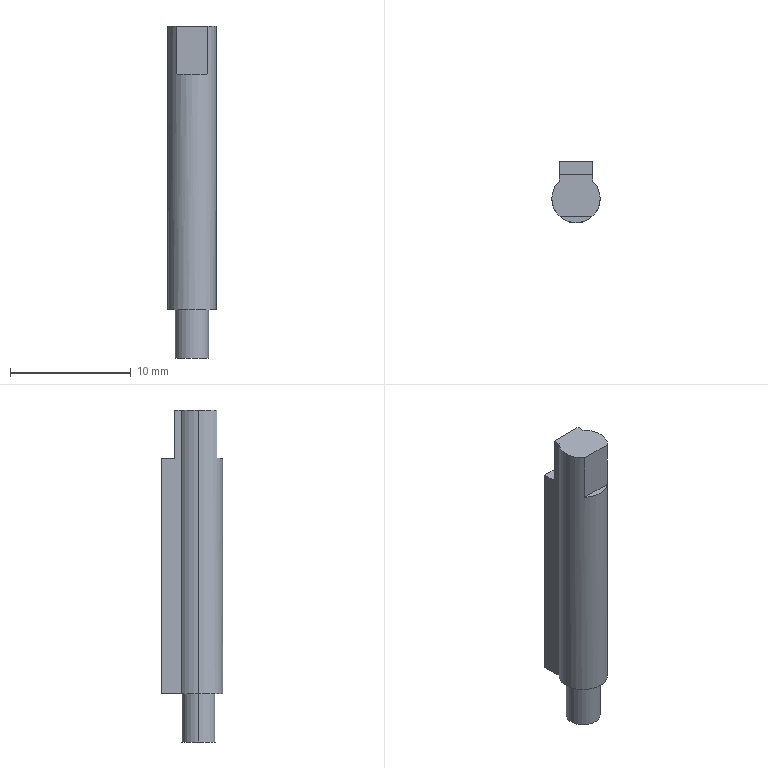Part | STEP file | QA-HI_MDX-SD_2 | 1 solid | 25 faces | box 4 x 5.1 x 27.5 mm | volume 387.922 mm3 | plane 16 | cylinder 7 | spline 2 | commonest cylinder face diameters 4 x3 2 x2 2.8 x2